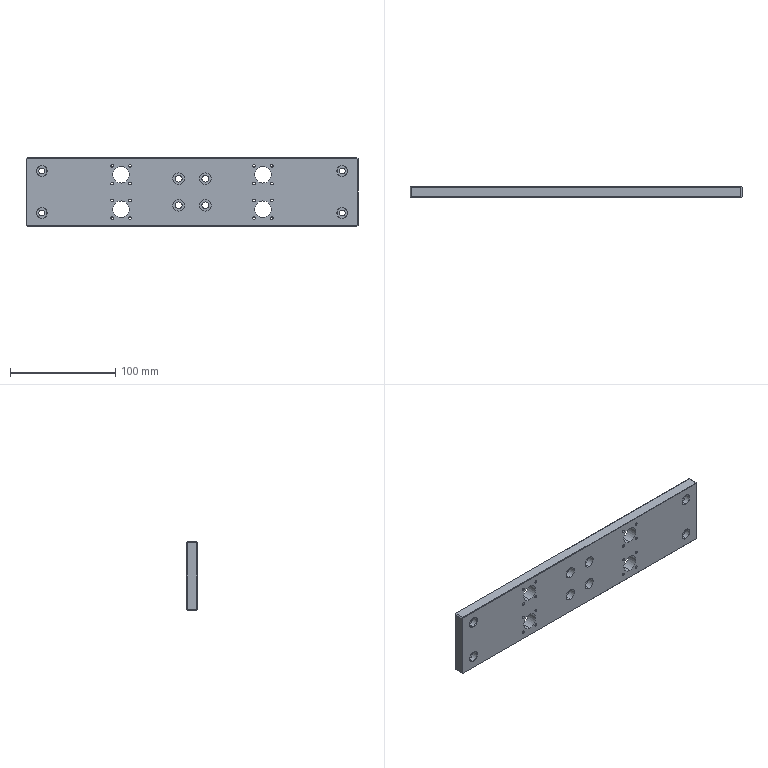Part | STEP file | lifting air cylinder fixing support seat 01 | 1 solid | 122 faces | box 316 x 10 x 65 mm | volume 191391 mm3 | cylinder 72 | plane 34 | cone 16 | commonest cylinder face diameters 2.5 x32 5.5 x8 6.6 x8 10 x8 11 x8 16 x8